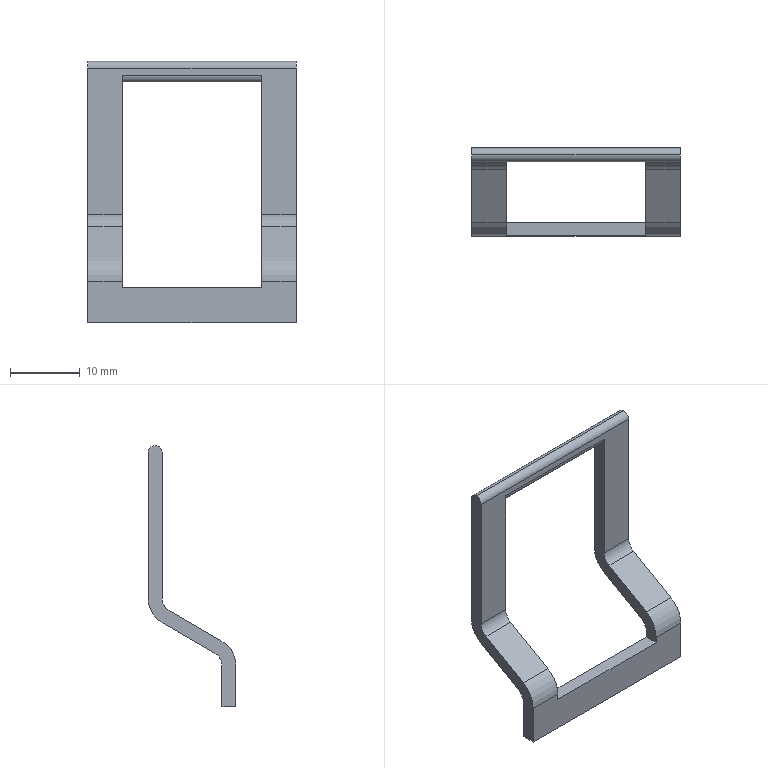Part | SolidWorks | features ICE 9, Draft 2, Fillet 2, Extrusion 1 | 1 solid | 25 faces | box 30 x 12.599 x 37.526 mm | volume 1159 mm3 | plane 14 | cylinder 11 | commonest cylinder face diameters 4 x4 8 x4 2 x3
STEP:
#1=CARTESIAN_POINT('',(0.,-2.,-1.));
#2=VERTEX_POINT('',#1);
#3=CARTESIAN_POINT('',(0.,-1.,0.));
#4=VERTEX_POINT('',#3);
#5=CARTESIAN_POINT('',(0.,-1.,-1.));
#6=DIRECTION('',(-1.,0.,0.));
#7=DIRECTION('',(0.,0.,1.));
#8=AXIS2_PLACEMENT_3D('',#5,#6,#7);
#9=CIRCLE('',#8,1.);
#10=EDGE_CURVE('',#2,#4,#9,.T.);
#11=ORIENTED_EDGE('',*,*,#10,.T.);
#12=CARTESIAN_POINT('',(-30.,-1.,0.));
#13=VERTEX_POINT('',#12);
#14=CARTESIAN_POINT('',(0.,-1.,0.));
#15=DIRECTION('',(-1.,0.,0.));
#16=VECTOR('',#15,1000.);
#17=LINE('',#14,#16);
#18=EDGE_CURVE('',#4,#13,#17,.T.);
#19=ORIENTED_EDGE('',*,*,#18,.T.);
#20=CARTESIAN_POINT('',(-30.,-2.,-1.));
#21=VERTEX_POINT('',#20);
#22=CARTESIAN_POINT('',(-30.,-1.,-1.));
#23=DIRECTION('',(-1.,0.,0.));
#24=DIRECTION('',(0.,0.,1.));
#25=AXIS2_PLACEMENT_3D('',#22,#23,#24);
#26=CIRCLE('',#25,1.);
#27=EDGE_CURVE('',#21,#13,#26,.T.);
#28=ORIENTED_EDGE('',*,*,#27,.F.);
#29=CARTESIAN_POINT('',(0.,-2.,-1.));
#30=DIRECTION('',(-1.,0.,0.));
#31=VECTOR('',#30,1000.);
#32=LINE('',#29,#31);
#33=EDGE_CURVE('',#2,#21,#32,.T.);
#34=ORIENTED_EDGE('',*,*,#33,.F.);
#35=EDGE_LOOP('',(#11,#19,#28,#34));
#36=FACE_OUTER_BOUND('',#35,.T.);
#37=CARTESIAN_POINT('',(0.,-1.,-1.));
#38=DIRECTION('',(-1.,0.,0.));
#39=DIRECTION('',(0.,0.,1.));
#40=AXIS2_PLACEMENT_3D('',#37,#38,#39);
#41=CYLINDRICAL_SURFACE('',#40,1.);
#42=ADVANCED_FACE('',(#36),#41,.T.);
#43=CARTESIAN_POINT('',(-5.,-2.,-2.));
#44=VERTEX_POINT('',#43);
#45=CARTESIAN_POINT('',(-25.,-2.,-2.));
#46=VERTEX_POINT('',#45);
#47=CARTESIAN_POINT('',(0.,-2.,-2.));
#48=DIRECTION('',(-1.,0.,0.));
#49=VECTOR('',#48,1000.);
#50=LINE('',#47,#49);
#51=EDGE_CURVE('',#44,#46,#50,.T.);
#52=ORIENTED_EDGE('',*,*,#51,.T.);
#53=CARTESIAN_POINT('',(-25.,0.,-2.));
#54=VERTEX_POINT('',#53);
#55=CARTESIAN_POINT('',(-25.,-1.,-2.));
#56=DIRECTION('',(-1.,0.,0.));
#57=DIRECTION('',(0.,0.,1.));
#58=AXIS2_PLACEMENT_3D('',#55,#56,#57);
#59=CIRCLE('',#58,1.);
#60=EDGE_CURVE('',#54,#46,#59,.T.);
#61=ORIENTED_EDGE('',*,*,#60,.F.);
#62=CARTESIAN_POINT('',(-5.,0.,-2.));
#63=VERTEX_POINT('',#62);
#64=CARTESIAN_POINT('',(0.,0.,-2.));
#65=DIRECTION('',(-1.,0.,0.));
#66=VECTOR('',#65,1000.);
#67=LINE('',#64,#66);
#68=EDGE_CURVE('',#63,#54,#67,.T.);
#69=ORIENTED_EDGE('',*,*,#68,.F.);
#70=CARTESIAN_POINT('',(-5.,-1.,-2.));
#71=DIRECTION('',(1.,0.,0.));
#72=DIRECTION('',(0.,0.,-1.));
#73=AXIS2_PLACEMENT_3D('',#70,#71,#72);
#74=CIRCLE('',#73,1.);
#75=EDGE_CURVE('',#44,#63,#74,.T.);
#76=ORIENTED_EDGE('',*,*,#75,.F.);
#77=EDGE_LOOP('',(#52,#61,#69,#76));
#78=FACE_OUTER_BOUND('',#77,.T.);
#79=CARTESIAN_POINT('',(0.,-1.,-2.));
#80=DIRECTION('',(-1.,0.,0.));
#81=DIRECTION('',(0.,0.,1.));
#82=AXIS2_PLACEMENT_3D('',#79,#80,#81);
#83=CYLINDRICAL_SURFACE('',#82,1.);
#84=ADVANCED_FACE('',(#78),#83,.T.);
#85=ORIENTED_EDGE('',*,*,#18,.F.);
#86=CARTESIAN_POINT('',(0.,0.,-1.));
#87=VERTEX_POINT('',#86);
#88=CARTESIAN_POINT('',(0.,-1.,-1.));
#89=DIRECTION('',(-1.,0.,0.));
#90=DIRECTION('',(0.,0.,1.));
#91=AXIS2_PLACEMENT_3D('',#88,#89,#90);
#92=CIRCLE('',#91,1.);
#93=EDGE_CURVE('',#4,#87,#92,.T.);
#94=ORIENTED_EDGE('',*,*,#93,.T.);
#95=CARTESIAN_POINT('',(-30.,0.,-1.));
#96=VERTEX_POINT('',#95);
#97=CARTESIAN_POINT('',(0.,0.,-1.));
#98=DIRECTION('',(-1.,0.,0.));
#99=VECTOR('',#98,1000.);
#100=LINE('',#97,#99);
#101=EDGE_CURVE('',#87,#96,#100,.T.);
#102=ORIENTED_EDGE('',*,*,#101,.T.);
#103=CARTESIAN_POINT('',(-30.,-1.,-1.));
#104=DIRECTION('',(-1.,0.,0.));
#105=DIRECTION('',(0.,0.,1.));
#106=AXIS2_PLACEMENT_3D('',#103,#104,#105);
#107=CIRCLE('',#106,1.);
#108=EDGE_CURVE('',#13,#96,#107,.T.);
#109=ORIENTED_EDGE('',*,*,#108,.F.);
#110=EDGE_LOOP('',(#85,#94,#102,#109));
#111=FACE_OUTER_BOUND('',#110,.T.);
#112=CARTESIAN_POINT('',(0.,-1.,-1.));
#113=DIRECTION('',(-1.,0.,0.));
#114=DIRECTION('',(0.,0.,1.));
#115=AXIS2_PLACEMENT_3D('',#112,#113,#114);
#116=CYLINDRICAL_SURFACE('',#115,1.);
#117=ADVANCED_FACE('',(#111),#116,.T.);
#118=CARTESIAN_POINT('',(-30.,-2.,-22.009));
#119=VERTEX_POINT('',#118);
#120=CARTESIAN_POINT('',(-30.,-2.,-2.));
#121=DIRECTION('',(0.,0.,1.));
#122=VECTOR('',#121,1000.);
#123=LINE('',#120,#122);
#124=EDGE_CURVE('',#119,#21,#123,.T.);
#125=ORIENTED_EDGE('',*,*,#124,.F.);
#126=CARTESIAN_POINT('',(-25.,-2.,-22.009));
#127=VERTEX_POINT('',#126);
#128=CARTESIAN_POINT('',(-25.,-2.,-22.009));
#129=DIRECTION('',(1.,0.,0.));
#130=VECTOR('',#129,1000.);
#131=LINE('',#128,#130);
#132=EDGE_CURVE('',#119,#127,#131,.T.);
#133=ORIENTED_EDGE('',*,*,#132,.T.);
#134=CARTESIAN_POINT('',(-25.,-2.,-3.));
#135=DIRECTION('',(0.,0.,1.));
#136=VECTOR('',#135,1000.);
#137=LINE('',#134,#136);
#138=EDGE_CURVE('',#127,#46,#137,.T.);
#139=ORIENTED_EDGE('',*,*,#138,.T.);
#140=ORIENTED_EDGE('',*,*,#51,.F.);
#141=CARTESIAN_POINT('',(-5.,-2.,-22.009));
#142=VERTEX_POINT('',#141);
#143=CARTESIAN_POINT('',(-5.,-2.,-3.));
#144=DIRECTION('',(0.,0.,1.));
#145=VECTOR('',#144,1000.);
#146=LINE('',#143,#145);
#147=EDGE_CURVE('',#142,#44,#146,.T.);
#148=ORIENTED_EDGE('',*,*,#147,.F.);
#149=CARTESIAN_POINT('',(0.,-2.,-22.009));
#150=VERTEX_POINT('',#149);
#151=CARTESIAN_POINT('',(0.,-2.,-22.009));
#152=DIRECTION('',(1.,0.,0.));
#153=VECTOR('',#152,1000.);
#154=LINE('',#151,#153);
#155=EDGE_CURVE('',#142,#150,#154,.T.);
#156=ORIENTED_EDGE('',*,*,#155,.T.);
#157=CARTESIAN_POINT('',(0.,-2.,-2.));
#158=DIRECTION('',(0.,0.,1.));
#159=VECTOR('',#158,1000.);
#160=LINE('',#157,#159);
#161=EDGE_CURVE('',#150,#2,#160,.T.);
#162=ORIENTED_EDGE('',*,*,#161,.T.);
#163=ORIENTED_EDGE('',*,*,#33,.T.);
#164=EDGE_LOOP('',(#125,#133,#139,#140,#148,#156,#162,#163));
#165=FACE_OUTER_BOUND('',#164,.T.);
#166=CARTESIAN_POINT('',(0.,-2.,-2.));
#167=DIRECTION('',(0.,-1.,0.));
#168=DIRECTION('',(0.,0.,-1.));
#169=AXIS2_PLACEMENT_3D('',#166,#167,#168);
#170=PLANE('',#169);
#171=ADVANCED_FACE('',(#165),#170,.T.);
#172=CARTESIAN_POINT('',(-25.,0.,-22.009));
#173=VERTEX_POINT('',#172);
#174=CARTESIAN_POINT('',(-25.,0.,-3.));
#175=DIRECTION('',(0.,0.,1.));
#176=VECTOR('',#175,1000.);
#177=LINE('',#174,#176);
#178=EDGE_CURVE('',#173,#54,#177,.T.);
#179=ORIENTED_EDGE('',*,*,#178,.F.);
#180=CARTESIAN_POINT('',(-30.,0.,-22.009));
#181=VERTEX_POINT('',#180);
#182=CARTESIAN_POINT('',(-30.,0.,-22.009));
#183=DIRECTION('',(-1.,0.,0.));
#184=VECTOR('',#183,1000.);
#185=LINE('',#182,#184);
#186=EDGE_CURVE('',#173,#181,#185,.T.);
#187=ORIENTED_EDGE('',*,*,#186,.T.);
#188=CARTESIAN_POINT('',(-30.,0.,-1.));
#189=DIRECTION('',(0.,0.,-1.));
#190=VECTOR('',#189,1000.);
#191=LINE('',#188,#190);
#192=EDGE_CURVE('',#96,#181,#191,.T.);
#193=ORIENTED_EDGE('',*,*,#192,.F.);
#194=ORIENTED_EDGE('',*,*,#101,.F.);
#195=CARTESIAN_POINT('',(0.,0.,-22.009));
#196=VERTEX_POINT('',#195);
#197=CARTESIAN_POINT('',(0.,0.,-1.));
#198=DIRECTION('',(0.,0.,-1.));
#199=VECTOR('',#198,1000.);
#200=LINE('',#197,#199);
#201=EDGE_CURVE('',#87,#196,#200,.T.);
#202=ORIENTED_EDGE('',*,*,#201,.T.);
#203=CARTESIAN_POINT('',(-5.,0.,-22.009));
#204=VERTEX_POINT('',#203);
#205=CARTESIAN_POINT('',(-5.,0.,-22.009));
#206=DIRECTION('',(-1.,0.,0.));
#207=VECTOR('',#206,1000.);
#208=LINE('',#205,#207);
#209=EDGE_CURVE('',#196,#204,#208,.T.);
#210=ORIENTED_EDGE('',*,*,#209,.T.);
#211=CARTESIAN_POINT('',(-5.,0.,-3.));
#212=DIRECTION('',(0.,0.,1.));
#213=VECTOR('',#212,1000.);
#214=LINE('',#211,#213);
#215=EDGE_CURVE('',#204,#63,#214,.T.);
#216=ORIENTED_EDGE('',*,*,#215,.T.);
#217=ORIENTED_EDGE('',*,*,#68,.T.);
#218=EDGE_LOOP('',(#179,#187,#193,#194,#202,#210,#216,#217));
#219=FACE_OUTER_BOUND('',#218,.T.);
#220=CARTESIAN_POINT('',(0.,0.,-1.));
#221=DIRECTION('',(0.,1.,0.));
#222=DIRECTION('',(0.,0.,1.));
#223=AXIS2_PLACEMENT_3D('',#220,#221,#222);
#224=PLANE('',#223);
#225=ADVANCED_FACE('',(#219),#224,.T.);
#226=CARTESIAN_POINT('',(0.,-2.,-25.473));
#227=VERTEX_POINT('',#226);
#228=CARTESIAN_POINT('',(0.,-9.599,-29.86));
#229=VERTEX_POINT('',#228);
#230=CARTESIAN_POINT('',(0.,0.,-24.318));
#231=DIRECTION('',(0.,-0.866,-0.5));
#232=VECTOR('',#231,1000.);
#233=LINE('',#230,#232);
#234=EDGE_CURVE('',#227,#229,#233,.T.);
#235=ORIENTED_EDGE('',*,*,#234,.F.);
#236=CARTESIAN_POINT('',(0.,-4.,-22.009));
#237=DIRECTION('',(1.,0.,0.));
#238=DIRECTION('',(0.,0.,1.));
#239=AXIS2_PLACEMENT_3D('',#236,#237,#238);
#240=CIRCLE('',#239,4.);
#241=EDGE_CURVE('',#227,#196,#240,.T.);
#242=ORIENTED_EDGE('',*,*,#241,.T.);
#243=ORIENTED_EDGE('',*,*,#201,.F.);
#244=ORIENTED_EDGE('',*,*,#93,.F.);
#245=ORIENTED_EDGE('',*,*,#10,.F.);
#246=ORIENTED_EDGE('',*,*,#161,.F.);
#247=CARTESIAN_POINT('',(0.,-3.,-23.741));
#248=VERTEX_POINT('',#247);
#249=CARTESIAN_POINT('',(0.,-4.,-22.009));
#250=DIRECTION('',(-1.,0.,0.));
#251=DIRECTION('',(0.,0.,1.));
#252=AXIS2_PLACEMENT_3D('',#249,#250,#251);
#253=CIRCLE('',#252,2.);
#254=EDGE_CURVE('',#150,#248,#253,.T.);
#255=ORIENTED_EDGE('',*,*,#254,.T.);
#256=CARTESIAN_POINT('',(0.,-10.599,-28.128));
#257=VERTEX_POINT('',#256);
#258=CARTESIAN_POINT('',(0.,-2.,-23.163));
#259=DIRECTION('',(0.,-0.866,-0.5));
#260=VECTOR('',#259,1000.);
#261=LINE('',#258,#260);
#262=EDGE_CURVE('',#248,#257,#261,.T.);
#263=ORIENTED_EDGE('',*,*,#262,.T.);
#264=CARTESIAN_POINT('',(0.,-12.599,-31.592));
#265=VERTEX_POINT('',#264);
#266=CARTESIAN_POINT('',(0.,-8.599,-31.592));
#267=DIRECTION('',(1.,0.,0.));
#268=DIRECTION('',(0.,0.,1.));
#269=AXIS2_PLACEMENT_3D('',#266,#267,#268);
#270=CIRCLE('',#269,4.);
#271=EDGE_CURVE('',#257,#265,#270,.T.);
#272=ORIENTED_EDGE('',*,*,#271,.T.);
#273=CARTESIAN_POINT('',(0.,-12.599,-37.526));
#274=VERTEX_POINT('',#273);
#275=CARTESIAN_POINT('',(0.,-12.599,-23.163));
#276=DIRECTION('',(0.,0.,1.));
#277=VECTOR('',#276,1000.);
#278=LINE('',#275,#277);
#279=EDGE_CURVE('',#274,#265,#278,.T.);
#280=ORIENTED_EDGE('',*,*,#279,.F.);
#281=CARTESIAN_POINT('',(0.,-10.599,-37.526));
#282=VERTEX_POINT('',#281);
#283=CARTESIAN_POINT('',(0.,-12.599,-37.526));
#284=DIRECTION('',(0.,1.,0.));
#285=VECTOR('',#284,1000.);
#286=LINE('',#283,#285);
#287=EDGE_CURVE('',#274,#282,#286,.T.);
#288=ORIENTED_EDGE('',*,*,#287,.T.);
#289=CARTESIAN_POINT('',(0.,-10.599,-31.592));
#290=VERTEX_POINT('',#289);
#291=CARTESIAN_POINT('',(0.,-10.599,-23.163));
#292=DIRECTION('',(0.,0.,1.));
#293=VECTOR('',#292,1000.);
#294=LINE('',#291,#293);
#295=EDGE_CURVE('',#282,#290,#294,.T.);
#296=ORIENTED_EDGE('',*,*,#295,.T.);
#297=CARTESIAN_POINT('',(0.,-8.599,-31.592));
#298=DIRECTION('',(-1.,0.,0.));
#299=DIRECTION('',(0.,0.,1.));
#300=AXIS2_PLACEMENT_3D('',#297,#298,#299);
#301=CIRCLE('',#300,2.);
#302=EDGE_CURVE('',#290,#229,#301,.T.);
#303=ORIENTED_EDGE('',*,*,#302,.T.);
#304=EDGE_LOOP('',(#235,#242,#243,#244,#245,#246,#255,#263,#272,#280,#288,#296,#303));
#305=FACE_OUTER_BOUND('',#304,.T.);
#306=CARTESIAN_POINT('',(0.,-1.,-1.));
#307=DIRECTION('',(-1.,0.,0.));
#308=DIRECTION('',(0.,0.,1.));
#309=AXIS2_PLACEMENT_3D('',#306,#307,#308);
#310=PLANE('',#309);
#311=ADVANCED_FACE('',(#305),#310,.F.);
#312=ORIENTED_EDGE('',*,*,#192,.T.);
#313=CARTESIAN_POINT('',(-30.,-2.,-25.473));
#314=VERTEX_POINT('',#313);
#315=CARTESIAN_POINT('',(-30.,-4.,-22.009));
#316=DIRECTION('',(-1.,0.,0.));
#317=DIRECTION('',(0.,0.,1.));
#318=AXIS2_PLACEMENT_3D('',#315,#316,#317);
#319=CIRCLE('',#318,4.);
#320=EDGE_CURVE('',#181,#314,#319,.T.);
#321=ORIENTED_EDGE('',*,*,#320,.T.);
#322=CARTESIAN_POINT('',(-30.,-9.599,-29.86));
#323=VERTEX_POINT('',#322);
#324=CARTESIAN_POINT('',(-30.,9.347,-18.922));
#325=DIRECTION('',(0.,0.866,0.5));
#326=VECTOR('',#325,1000.);
#327=LINE('',#324,#326);
#328=EDGE_CURVE('',#323,#314,#327,.T.);
#329=ORIENTED_EDGE('',*,*,#328,.F.);
#330=CARTESIAN_POINT('',(-30.,-10.599,-31.592));
#331=VERTEX_POINT('',#330);
#332=CARTESIAN_POINT('',(-30.,-8.599,-31.592));
#333=DIRECTION('',(1.,0.,0.));
#334=DIRECTION('',(0.,0.,1.));
#335=AXIS2_PLACEMENT_3D('',#332,#333,#334);
#336=CIRCLE('',#335,2.);
#337=EDGE_CURVE('',#323,#331,#336,.T.);
#338=ORIENTED_EDGE('',*,*,#337,.T.);
#339=CARTESIAN_POINT('',(-30.,-10.599,-37.526));
#340=VERTEX_POINT('',#339);
#341=CARTESIAN_POINT('',(-30.,-10.599,-37.526));
#342=DIRECTION('',(0.,0.,-1.));
#343=VECTOR('',#342,1000.);
#344=LINE('',#341,#343);
#345=EDGE_CURVE('',#331,#340,#344,.T.);
#346=ORIENTED_EDGE('',*,*,#345,.T.);
#347=CARTESIAN_POINT('',(-30.,-12.599,-37.526));
#348=VERTEX_POINT('',#347);
#349=CARTESIAN_POINT('',(-30.,-12.599,-37.526));
#350=DIRECTION('',(0.,1.,0.));
#351=VECTOR('',#350,1000.);
#352=LINE('',#349,#351);
#353=EDGE_CURVE('',#348,#340,#352,.T.);
#354=ORIENTED_EDGE('',*,*,#353,.F.);
#355=CARTESIAN_POINT('',(-30.,-12.599,-31.592));
#356=VERTEX_POINT('',#355);
#357=CARTESIAN_POINT('',(-30.,-12.599,-37.526));
#358=DIRECTION('',(0.,0.,-1.));
#359=VECTOR('',#358,1000.);
#360=LINE('',#357,#359);
#361=EDGE_CURVE('',#356,#348,#360,.T.);
#362=ORIENTED_EDGE('',*,*,#361,.F.);
#363=CARTESIAN_POINT('',(-30.,-10.599,-28.128));
#364=VERTEX_POINT('',#363);
#365=CARTESIAN_POINT('',(-30.,-8.599,-31.592));
#366=DIRECTION('',(-1.,0.,0.));
#367=DIRECTION('',(0.,0.,1.));
#368=AXIS2_PLACEMENT_3D('',#365,#366,#367);
#369=CIRCLE('',#368,4.);
#370=EDGE_CURVE('',#356,#364,#369,.T.);
#371=ORIENTED_EDGE('',*,*,#370,.T.);
#372=CARTESIAN_POINT('',(-30.,-3.,-23.741));
#373=VERTEX_POINT('',#372);
#374=CARTESIAN_POINT('',(-30.,8.347,-17.19));
#375=DIRECTION('',(0.,0.866,0.5));
#376=VECTOR('',#375,1000.);
#377=LINE('',#374,#376);
#378=EDGE_CURVE('',#364,#373,#377,.T.);
#379=ORIENTED_EDGE('',*,*,#378,.T.);
#380=CARTESIAN_POINT('',(-30.,-4.,-22.009));
#381=DIRECTION('',(1.,0.,0.));
#382=DIRECTION('',(0.,0.,1.));
#383=AXIS2_PLACEMENT_3D('',#380,#381,#382);
#384=CIRCLE('',#383,2.);
#385=EDGE_CURVE('',#373,#119,#384,.T.);
#386=ORIENTED_EDGE('',*,*,#385,.T.);
#387=ORIENTED_EDGE('',*,*,#124,.T.);
#388=ORIENTED_EDGE('',*,*,#27,.T.);
#389=ORIENTED_EDGE('',*,*,#108,.T.);
#390=EDGE_LOOP('',(#312,#321,#329,#338,#346,#354,#362,#371,#379,#386,#387,#388,#389));
#391=FACE_OUTER_BOUND('',#390,.T.);
#392=CARTESIAN_POINT('',(-30.,-1.,-1.));
#393=DIRECTION('',(-1.,0.,0.));
#394=DIRECTION('',(0.,0.,1.));
#395=AXIS2_PLACEMENT_3D('',#392,#393,#394);
#396=PLANE('',#395);
#397=ADVANCED_FACE('',(#391),#396,.T.);
#398=ORIENTED_EDGE('',*,*,#215,.F.);
#399=CARTESIAN_POINT('',(-5.,-2.,-25.473));
#400=VERTEX_POINT('',#399);
#401=CARTESIAN_POINT('',(-5.,-4.,-22.009));
#402=DIRECTION('',(-1.,0.,0.));
#403=DIRECTION('',(0.,0.,-1.));
#404=AXIS2_PLACEMENT_3D('',#401,#402,#403);
#405=CIRCLE('',#404,4.);
#406=EDGE_CURVE('',#204,#400,#405,.T.);
#407=ORIENTED_EDGE('',*,*,#406,.T.);
#408=CARTESIAN_POINT('',(-5.,-9.599,-29.86));
#409=VERTEX_POINT('',#408);
#410=CARTESIAN_POINT('',(-5.,0.,-24.318));
#411=DIRECTION('',(0.,0.866,0.5));
#412=VECTOR('',#411,1000.);
#413=LINE('',#410,#412);
#414=EDGE_CURVE('',#409,#400,#413,.T.);
#415=ORIENTED_EDGE('',*,*,#414,.F.);
#416=CARTESIAN_POINT('',(-5.,-10.599,-31.592));
#417=VERTEX_POINT('',#416);
#418=CARTESIAN_POINT('',(-5.,-8.599,-31.592));
#419=DIRECTION('',(1.,0.,0.));
#420=DIRECTION('',(0.,0.,-1.));
#421=AXIS2_PLACEMENT_3D('',#418,#419,#420);
#422=CIRCLE('',#421,2.);
#423=EDGE_CURVE('',#409,#417,#422,.T.);
#424=ORIENTED_EDGE('',*,*,#423,.T.);
#425=CARTESIAN_POINT('',(-5.,-10.599,-32.526));
#426=VERTEX_POINT('',#425);
#427=CARTESIAN_POINT('',(-5.,-10.599,-32.526));
#428=DIRECTION('',(0.,0.,-1.));
#429=VECTOR('',#428,1000.);
#430=LINE('',#427,#429);
#431=EDGE_CURVE('',#417,#426,#430,.T.);
#432=ORIENTED_EDGE('',*,*,#431,.T.);
#433=CARTESIAN_POINT('',(-5.,-12.599,-32.526));
#434=VERTEX_POINT('',#433);
#435=CARTESIAN_POINT('',(-5.,-12.599,-32.526));
#436=DIRECTION('',(0.,1.,0.));
#437=VECTOR('',#436,1000.);
#438=LINE('',#435,#437);
#439=EDGE_CURVE('',#434,#426,#438,.T.);
#440=ORIENTED_EDGE('',*,*,#439,.F.);
#441=CARTESIAN_POINT('',(-5.,-12.599,-31.592));
#442=VERTEX_POINT('',#441);
#443=CARTESIAN_POINT('',(-5.,-12.599,-32.526));
#444=DIRECTION('',(0.,0.,-1.));
#445=VECTOR('',#444,1000.);
#446=LINE('',#443,#445);
#447=EDGE_CURVE('',#442,#434,#446,.T.);
#448=ORIENTED_EDGE('',*,*,#447,.F.);
#449=CARTESIAN_POINT('',(-5.,-10.599,-28.128));
#450=VERTEX_POINT('',#449);
#451=CARTESIAN_POINT('',(-5.,-8.599,-31.592));
#452=DIRECTION('',(-1.,0.,0.));
#453=DIRECTION('',(0.,0.,-1.));
#454=AXIS2_PLACEMENT_3D('',#451,#452,#453);
#455=CIRCLE('',#454,4.);
#456=EDGE_CURVE('',#442,#450,#455,.T.);
#457=ORIENTED_EDGE('',*,*,#456,.T.);
#458=CARTESIAN_POINT('',(-5.,-3.,-23.741));
#459=VERTEX_POINT('',#458);
#460=CARTESIAN_POINT('',(-5.,-2.,-23.163));
#461=DIRECTION('',(0.,0.866,0.5));
#462=VECTOR('',#461,1000.);
#463=LINE('',#460,#462);
#464=EDGE_CURVE('',#450,#459,#463,.T.);
#465=ORIENTED_EDGE('',*,*,#464,.T.);
#466=CARTESIAN_POINT('',(-5.,-4.,-22.009));
#467=DIRECTION('',(1.,0.,0.));
#468=DIRECTION('',(0.,0.,-1.));
#469=AXIS2_PLACEMENT_3D('',#466,#467,#468);
#470=CIRCLE('',#469,2.);
#471=EDGE_CURVE('',#459,#142,#470,.T.);
#472=ORIENTED_EDGE('',*,*,#471,.T.);
#473=ORIENTED_EDGE('',*,*,#147,.T.);
#474=ORIENTED_EDGE('',*,*,#75,.T.);
#475=EDGE_LOOP('',(#398,#407,#415,#424,#432,#440,#448,#457,#465,#472,#473,#474));
#476=FACE_OUTER_BOUND('',#475,.T.);
#477=CARTESIAN_POINT('',(-5.,0.,-3.));
#478=DIRECTION('',(1.,0.,0.));
#479=DIRECTION('',(0.,0.,-1.));
#480=AXIS2_PLACEMENT_3D('',#477,#478,#479);
#481=PLANE('',#480);
#482=ADVANCED_FACE('',(#476),#481,.F.);
#483=ORIENTED_EDGE('',*,*,#414,.T.);
#484=CARTESIAN_POINT('',(0.,-2.,-25.473));
#485=DIRECTION('',(1.,0.,0.));
#486=VECTOR('',#485,1000.);
#487=LINE('',#484,#486);
#488=EDGE_CURVE('',#400,#227,#487,.T.);
#489=ORIENTED_EDGE('',*,*,#488,.T.);
#490=ORIENTED_EDGE('',*,*,#234,.T.);
#491=CARTESIAN_POINT('',(0.,-9.599,-29.86));
#492=DIRECTION('',(-1.,0.,0.));
#493=VECTOR('',#492,1000.);
#494=LINE('',#491,#493);
#495=EDGE_CURVE('',#229,#409,#494,.T.);
#496=ORIENTED_EDGE('',*,*,#495,.T.);
#497=EDGE_LOOP('',(#483,#489,#490,#496));
#498=FACE_OUTER_BOUND('',#497,.T.);
#499=CARTESIAN_POINT('',(0.,0.,-24.318));
#500=DIRECTION('',(0.,0.5,-0.866));
#501=DIRECTION('',(0.,0.866,0.5));
#502=AXIS2_PLACEMENT_3D('',#499,#500,#501);
#503=PLANE('',#502);
#504=ADVANCED_FACE('',(#498),#503,.T.);
#505=ORIENTED_EDGE('',*,*,#464,.F.);
#506=CARTESIAN_POINT('',(0.,-10.599,-28.128));
#507=DIRECTION('',(1.,0.,0.));
#508=VECTOR('',#507,1000.);
#509=LINE('',#506,#508);
#510=EDGE_CURVE('',#450,#257,#509,.T.);
#511=ORIENTED_EDGE('',*,*,#510,.T.);
#512=ORIENTED_EDGE('',*,*,#262,.F.);
#513=CARTESIAN_POINT('',(-5.,-3.,-23.741));
#514=DIRECTION('',(-1.,0.,0.));
#515=VECTOR('',#514,1000.);
#516=LINE('',#513,#515);
#517=EDGE_CURVE('',#248,#459,#516,.T.);
#518=ORIENTED_EDGE('',*,*,#517,.T.);
#519=EDGE_LOOP('',(#505,#511,#512,#518));
#520=FACE_OUTER_BOUND('',#519,.T.);
#521=CARTESIAN_POINT('',(-5.,-2.,-23.163));
#522=DIRECTION('',(0.,-0.5,0.866));
#523=DIRECTION('',(0.,-0.866,-0.5));
#524=AXIS2_PLACEMENT_3D('',#521,#522,#523);
#525=PLANE('',#524);
#526=ADVANCED_FACE('',(#520),#525,.T.);
#527=CARTESIAN_POINT('',(-25.,-2.,-25.473));
#528=VERTEX_POINT('',#527);
#529=CARTESIAN_POINT('',(-25.,-9.599,-29.86));
#530=VERTEX_POINT('',#529);
#531=CARTESIAN_POINT('',(-25.,0.,-24.318));
#532=DIRECTION('',(0.,-0.866,-0.5));
#533=VECTOR('',#532,1000.);
#534=LINE('',#531,#533);
#535=EDGE_CURVE('',#528,#530,#534,.T.);
#536=ORIENTED_EDGE('',*,*,#535,.F.);
#537=CARTESIAN_POINT('',(-25.,-4.,-22.009));
#538=DIRECTION('',(1.,0.,0.));
#539=DIRECTION('',(0.,0.,1.));
#540=AXIS2_PLACEMENT_3D('',#537,#538,#539);
#541=CIRCLE('',#540,4.);
#542=EDGE_CURVE('',#528,#173,#541,.T.);
#543=ORIENTED_EDGE('',*,*,#542,.T.);
#544=ORIENTED_EDGE('',*,*,#178,.T.);
#545=ORIENTED_EDGE('',*,*,#60,.T.);
#546=ORIENTED_EDGE('',*,*,#138,.F.);
#547=CARTESIAN_POINT('',(-25.,-3.,-23.741));
#548=VERTEX_POINT('',#547);
#549=CARTESIAN_POINT('',(-25.,-4.,-22.009));
#550=DIRECTION('',(-1.,0.,0.));
#551=DIRECTION('',(0.,0.,1.));
#552=AXIS2_PLACEMENT_3D('',#549,#550,#551);
#553=CIRCLE('',#552,2.);
#554=EDGE_CURVE('',#127,#548,#553,.T.);
#555=ORIENTED_EDGE('',*,*,#554,.T.);
#556=CARTESIAN_POINT('',(-25.,-10.599,-28.128));
#557=VERTEX_POINT('',#556);
#558=CARTESIAN_POINT('',(-25.,-2.,-23.163));
#559=DIRECTION('',(0.,-0.866,-0.5));
#560=VECTOR('',#559,1000.);
#561=LINE('',#558,#560);
#562=EDGE_CURVE('',#548,#557,#561,.T.);
#563=ORIENTED_EDGE('',*,*,#562,.T.);
#564=CARTESIAN_POINT('',(-25.,-12.599,-31.592));
#565=VERTEX_POINT('',#564);
#566=CARTESIAN_POINT('',(-25.,-8.599,-31.592));
#567=DIRECTION('',(1.,0.,0.));
#568=DIRECTION('',(0.,0.,1.));
#569=AXIS2_PLACEMENT_3D('',#566,#567,#568);
#570=CIRCLE('',#569,4.);
#571=EDGE_CURVE('',#557,#565,#570,.T.);
#572=ORIENTED_EDGE('',*,*,#571,.T.);
#573=CARTESIAN_POINT('',(-25.,-12.599,-32.526));
#574=VERTEX_POINT('',#573);
#575=CARTESIAN_POINT('',(-25.,-12.599,-23.163));
#576=DIRECTION('',(0.,0.,1.));
#577=VECTOR('',#576,1000.);
#578=LINE('',#575,#577);
#579=EDGE_CURVE('',#574,#565,#578,.T.);
#580=ORIENTED_EDGE('',*,*,#579,.F.);
#581=CARTESIAN_POINT('',(-25.,-10.599,-32.526));
#582=VERTEX_POINT('',#581);
#583=CARTESIAN_POINT('',(-25.,-12.599,-32.526));
#584=DIRECTION('',(0.,1.,0.));
#585=VECTOR('',#584,1000.);
#586=LINE('',#583,#585);
#587=EDGE_CURVE('',#574,#582,#586,.T.);
#588=ORIENTED_EDGE('',*,*,#587,.T.);
#589=CARTESIAN_POINT('',(-25.,-10.599,-31.592));
#590=VERTEX_POINT('',#589);
#591=CARTESIAN_POINT('',(-25.,-10.599,-23.163));
#592=DIRECTION('',(0.,0.,1.));
#593=VECTOR('',#592,1000.);
#594=LINE('',#591,#593);
#595=EDGE_CURVE('',#582,#590,#594,.T.);
#596=ORIENTED_EDGE('',*,*,#595,.T.);
#597=CARTESIAN_POINT('',(-25.,-8.599,-31.592));
#598=DIRECTION('',(-1.,0.,0.));
#599=DIRECTION('',(0.,0.,1.));
#600=AXIS2_PLACEMENT_3D('',#597,#598,#599);
#601=CIRCLE('',#600,2.);
#602=EDGE_CURVE('',#590,#530,#601,.T.);
#603=ORIENTED_EDGE('',*,*,#602,.T.);
#604=EDGE_LOOP('',(#536,#543,#544,#545,#546,#555,#563,#572,#580,#588,#596,#603));
#605=FACE_OUTER_BOUND('',#604,.T.);
#606=CARTESIAN_POINT('',(-25.,-2.,-3.));
#607=DIRECTION('',(-1.,0.,0.));
#608=DIRECTION('',(0.,0.,1.));
#609=AXIS2_PLACEMENT_3D('',#606,#607,#608);
#610=PLANE('',#609);
#611=ADVANCED_FACE('',(#605),#610,.F.);
#612=ORIENTED_EDGE('',*,*,#328,.T.);
#613=CARTESIAN_POINT('',(-25.,-2.,-25.473));
#614=DIRECTION('',(1.,0.,0.));
#615=VECTOR('',#614,1000.);
#616=LINE('',#613,#615);
#617=EDGE_CURVE('',#314,#528,#616,.T.);
#618=ORIENTED_EDGE('',*,*,#617,.T.);
#619=ORIENTED_EDGE('',*,*,#535,.T.);
#620=CARTESIAN_POINT('',(-25.,-9.599,-29.86));
#621=DIRECTION('',(-1.,0.,0.));
#622=VECTOR('',#621,1000.);
#623=LINE('',#620,#622);
#624=EDGE_CURVE('',#530,#323,#623,.T.);
#625=ORIENTED_EDGE('',*,*,#624,.T.);
#626=EDGE_LOOP('',(#612,#618,#619,#625));
#627=FACE_OUTER_BOUND('',#626,.T.);
#628=CARTESIAN_POINT('',(-25.,0.,-24.318));
#629=DIRECTION('',(0.,0.5,-0.866));
#630=DIRECTION('',(0.,0.866,0.5));
#631=AXIS2_PLACEMENT_3D('',#628,#629,#630);
#632=PLANE('',#631);
#633=ADVANCED_FACE('',(#627),#632,.T.);
#634=ORIENTED_EDGE('',*,*,#378,.F.);
#635=CARTESIAN_POINT('',(-25.,-10.599,-28.128));
#636=DIRECTION('',(1.,0.,0.));
#637=VECTOR('',#636,1000.);
#638=LINE('',#635,#637);
#639=EDGE_CURVE('',#364,#557,#638,.T.);
#640=ORIENTED_EDGE('',*,*,#639,.T.);
#641=ORIENTED_EDGE('',*,*,#562,.F.);
#642=CARTESIAN_POINT('',(-30.,-3.,-23.741));
#643=DIRECTION('',(-1.,0.,0.));
#644=VECTOR('',#643,1000.);
#645=LINE('',#642,#644);
#646=EDGE_CURVE('',#548,#373,#645,.T.);
#647=ORIENTED_EDGE('',*,*,#646,.T.);
#648=EDGE_LOOP('',(#634,#640,#641,#647));
#649=FACE_OUTER_BOUND('',#648,.T.);
#650=CARTESIAN_POINT('',(-30.,-2.,-23.163));
#651=DIRECTION('',(0.,-0.5,0.866));
#652=DIRECTION('',(0.,-0.866,-0.5));
#653=AXIS2_PLACEMENT_3D('',#650,#651,#652);
#654=PLANE('',#653);
#655=ADVANCED_FACE('',(#649),#654,.T.);
#656=ORIENTED_EDGE('',*,*,#345,.F.);
#657=CARTESIAN_POINT('',(0.,-10.599,-31.592));
#658=DIRECTION('',(1.,0.,0.));
#659=VECTOR('',#658,1000.);
#660=LINE('',#657,#659);
#661=EDGE_CURVE('',#331,#590,#660,.T.);
#662=ORIENTED_EDGE('',*,*,#661,.T.);
#663=ORIENTED_EDGE('',*,*,#595,.F.);
#664=CARTESIAN_POINT('',(-25.,-10.599,-32.526));
#665=DIRECTION('',(-1.,0.,0.));
#666=VECTOR('',#665,1000.);
#667=LINE('',#664,#666);
#668=EDGE_CURVE('',#426,#582,#667,.T.);
#669=ORIENTED_EDGE('',*,*,#668,.F.);
#670=ORIENTED_EDGE('',*,*,#431,.F.);
#671=CARTESIAN_POINT('',(0.,-10.599,-31.592));
#672=DIRECTION('',(1.,0.,0.));
#673=VECTOR('',#672,1000.);
#674=LINE('',#671,#673);
#675=EDGE_CURVE('',#417,#290,#674,.T.);
#676=ORIENTED_EDGE('',*,*,#675,.T.);
#677=ORIENTED_EDGE('',*,*,#295,.F.);
#678=CARTESIAN_POINT('',(0.,-10.599,-37.526));
#679=DIRECTION('',(1.,0.,0.));
#680=VECTOR('',#679,1000.);
#681=LINE('',#678,#680);
#682=EDGE_CURVE('',#340,#282,#681,.T.);
#683=ORIENTED_EDGE('',*,*,#682,.F.);
#684=EDGE_LOOP('',(#656,#662,#663,#669,#670,#676,#677,#683));
#685=FACE_OUTER_BOUND('',#684,.T.);
#686=CARTESIAN_POINT('',(0.,-10.599,0.));
#687=DIRECTION('',(0.,1.,0.));
#688=DIRECTION('',(0.,0.,1.));
#689=AXIS2_PLACEMENT_3D('',#686,#687,#688);
#690=PLANE('',#689);
#691=ADVANCED_FACE('',(#685),#690,.T.);
#692=ORIENTED_EDGE('',*,*,#668,.T.);
#693=ORIENTED_EDGE('',*,*,#587,.F.);
#694=CARTESIAN_POINT('',(-25.,-12.599,-32.526));
#695=DIRECTION('',(-1.,0.,0.));
#696=VECTOR('',#695,1000.);
#697=LINE('',#694,#696);
#698=EDGE_CURVE('',#434,#574,#697,.T.);
#699=ORIENTED_EDGE('',*,*,#698,.F.);
#700=ORIENTED_EDGE('',*,*,#439,.T.);
#701=EDGE_LOOP('',(#692,#693,#699,#700));
#702=FACE_OUTER_BOUND('',#701,.T.);
#703=CARTESIAN_POINT('',(-25.,-12.599,-32.526));
#704=DIRECTION('',(0.,0.,-1.));
#705=DIRECTION('',(-1.,0.,0.));
#706=AXIS2_PLACEMENT_3D('',#703,#704,#705);
#707=PLANE('',#706);
#708=ADVANCED_FACE('',(#702),#707,.F.);
#709=ORIENTED_EDGE('',*,*,#682,.T.);
#710=ORIENTED_EDGE('',*,*,#287,.F.);
#711=CARTESIAN_POINT('',(0.,-12.599,-37.526));
#712=DIRECTION('',(1.,0.,0.));
#713=VECTOR('',#712,1000.);
#714=LINE('',#711,#713);
#715=EDGE_CURVE('',#348,#274,#714,.T.);
#716=ORIENTED_EDGE('',*,*,#715,.F.);
#717=ORIENTED_EDGE('',*,*,#353,.T.);
#718=EDGE_LOOP('',(#709,#710,#716,#717));
#719=FACE_OUTER_BOUND('',#718,.T.);
#720=CARTESIAN_POINT('',(0.,-12.599,-37.526));
#721=DIRECTION('',(0.,0.,1.));
#722=DIRECTION('',(1.,0.,0.));
#723=AXIS2_PLACEMENT_3D('',#720,#721,#722);
#724=PLANE('',#723);
#725=ADVANCED_FACE('',(#719),#724,.F.);
#726=ORIENTED_EDGE('',*,*,#279,.T.);
#727=CARTESIAN_POINT('',(-5.,-12.599,-31.592));
#728=DIRECTION('',(-1.,0.,0.));
#729=VECTOR('',#728,1000.);
#730=LINE('',#727,#729);
#731=EDGE_CURVE('',#265,#442,#730,.T.);
#732=ORIENTED_EDGE('',*,*,#731,.T.);
#733=ORIENTED_EDGE('',*,*,#447,.T.);
#734=ORIENTED_EDGE('',*,*,#698,.T.);
#735=ORIENTED_EDGE('',*,*,#579,.T.);
#736=CARTESIAN_POINT('',(-30.,-12.599,-31.592));
#737=DIRECTION('',(-1.,0.,0.));
#738=VECTOR('',#737,1000.);
#739=LINE('',#736,#738);
#740=EDGE_CURVE('',#565,#356,#739,.T.);
#741=ORIENTED_EDGE('',*,*,#740,.T.);
#742=ORIENTED_EDGE('',*,*,#361,.T.);
#743=ORIENTED_EDGE('',*,*,#715,.T.);
#744=EDGE_LOOP('',(#726,#732,#733,#734,#735,#741,#742,#743));
#745=FACE_OUTER_BOUND('',#744,.T.);
#746=CARTESIAN_POINT('',(0.,-12.599,0.));
#747=DIRECTION('',(0.,1.,0.));
#748=DIRECTION('',(0.,0.,1.));
#749=AXIS2_PLACEMENT_3D('',#746,#747,#748);
#750=PLANE('',#749);
#751=ADVANCED_FACE('',(#745),#750,.F.);
#752=ORIENTED_EDGE('',*,*,#554,.F.);
#753=ORIENTED_EDGE('',*,*,#132,.F.);
#754=ORIENTED_EDGE('',*,*,#385,.F.);
#755=ORIENTED_EDGE('',*,*,#646,.F.);
#756=EDGE_LOOP('',(#752,#753,#754,#755));
#757=FACE_OUTER_BOUND('',#756,.T.);
#758=CARTESIAN_POINT('',(-30.,-4.,-22.009));
#759=DIRECTION('',(1.,0.,0.));
#760=DIRECTION('',(0.,0.,-1.));
#761=AXIS2_PLACEMENT_3D('',#758,#759,#760);
#762=CYLINDRICAL_SURFACE('',#761,2.);
#763=ADVANCED_FACE('',(#757),#762,.F.);
#764=ORIENTED_EDGE('',*,*,#254,.F.);
#765=ORIENTED_EDGE('',*,*,#155,.F.);
#766=ORIENTED_EDGE('',*,*,#471,.F.);
#767=ORIENTED_EDGE('',*,*,#517,.F.);
#768=EDGE_LOOP('',(#764,#765,#766,#767));
#769=FACE_OUTER_BOUND('',#768,.T.);
#770=CARTESIAN_POINT('',(-5.,-4.,-22.009));
#771=DIRECTION('',(1.,0.,0.));
#772=DIRECTION('',(0.,0.,-1.));
#773=AXIS2_PLACEMENT_3D('',#770,#771,#772);
#774=CYLINDRICAL_SURFACE('',#773,2.);
#775=ADVANCED_FACE('',(#769),#774,.F.);
#776=ORIENTED_EDGE('',*,*,#602,.F.);
#777=ORIENTED_EDGE('',*,*,#661,.F.);
#778=ORIENTED_EDGE('',*,*,#337,.F.);
#779=ORIENTED_EDGE('',*,*,#624,.F.);
#780=EDGE_LOOP('',(#776,#777,#778,#779));
#781=FACE_OUTER_BOUND('',#780,.T.);
#782=CARTESIAN_POINT('',(-25.,-8.599,-31.592));
#783=DIRECTION('',(1.,0.,0.));
#784=DIRECTION('',(0.,0.,-1.));
#785=AXIS2_PLACEMENT_3D('',#782,#783,#784);
#786=CYLINDRICAL_SURFACE('',#785,2.);
#787=ADVANCED_FACE('',(#781),#786,.F.);
#788=ORIENTED_EDGE('',*,*,#302,.F.);
#789=ORIENTED_EDGE('',*,*,#675,.F.);
#790=ORIENTED_EDGE('',*,*,#423,.F.);
#791=ORIENTED_EDGE('',*,*,#495,.F.);
#792=EDGE_LOOP('',(#788,#789,#790,#791));
#793=FACE_OUTER_BOUND('',#792,.T.);
#794=CARTESIAN_POINT('',(0.,-8.599,-31.592));
#795=DIRECTION('',(1.,0.,0.));
#796=DIRECTION('',(0.,0.,-1.));
#797=AXIS2_PLACEMENT_3D('',#794,#795,#796);
#798=CYLINDRICAL_SURFACE('',#797,2.);
#799=ADVANCED_FACE('',(#793),#798,.F.);
#800=ORIENTED_EDGE('',*,*,#320,.F.);
#801=ORIENTED_EDGE('',*,*,#186,.F.);
#802=ORIENTED_EDGE('',*,*,#542,.F.);
#803=ORIENTED_EDGE('',*,*,#617,.F.);
#804=EDGE_LOOP('',(#800,#801,#802,#803));
#805=FACE_OUTER_BOUND('',#804,.T.);
#806=CARTESIAN_POINT('',(-25.,-4.,-22.009));
#807=DIRECTION('',(1.,0.,0.));
#808=DIRECTION('',(0.,0.,-1.));
#809=AXIS2_PLACEMENT_3D('',#806,#807,#808);
#810=CYLINDRICAL_SURFACE('',#809,4.);
#811=ADVANCED_FACE('',(#805),#810,.T.);
#812=ORIENTED_EDGE('',*,*,#406,.F.);
#813=ORIENTED_EDGE('',*,*,#209,.F.);
#814=ORIENTED_EDGE('',*,*,#241,.F.);
#815=ORIENTED_EDGE('',*,*,#488,.F.);
#816=EDGE_LOOP('',(#812,#813,#814,#815));
#817=FACE_OUTER_BOUND('',#816,.T.);
#818=CARTESIAN_POINT('',(0.,-4.,-22.009));
#819=DIRECTION('',(1.,0.,0.));
#820=DIRECTION('',(0.,0.,-1.));
#821=AXIS2_PLACEMENT_3D('',#818,#819,#820);
#822=CYLINDRICAL_SURFACE('',#821,4.);
#823=ADVANCED_FACE('',(#817),#822,.T.);
#824=ORIENTED_EDGE('',*,*,#271,.F.);
#825=ORIENTED_EDGE('',*,*,#510,.F.);
#826=ORIENTED_EDGE('',*,*,#456,.F.);
#827=ORIENTED_EDGE('',*,*,#731,.F.);
#828=EDGE_LOOP('',(#824,#825,#826,#827));
#829=FACE_OUTER_BOUND('',#828,.T.);
#830=CARTESIAN_POINT('',(0.,-8.599,-31.592));
#831=DIRECTION('',(1.,0.,0.));
#832=DIRECTION('',(0.,0.,-1.));
#833=AXIS2_PLACEMENT_3D('',#830,#831,#832);
#834=CYLINDRICAL_SURFACE('',#833,4.);
#835=ADVANCED_FACE('',(#829),#834,.T.);
#836=ORIENTED_EDGE('',*,*,#571,.F.);
#837=ORIENTED_EDGE('',*,*,#639,.F.);
#838=ORIENTED_EDGE('',*,*,#370,.F.);
#839=ORIENTED_EDGE('',*,*,#740,.F.);
#840=EDGE_LOOP('',(#836,#837,#838,#839));
#841=FACE_OUTER_BOUND('',#840,.T.);
#842=CARTESIAN_POINT('',(0.,-8.599,-31.592));
#843=DIRECTION('',(1.,0.,0.));
#844=DIRECTION('',(0.,0.,-1.));
#845=AXIS2_PLACEMENT_3D('',#842,#843,#844);
#846=CYLINDRICAL_SURFACE('',#845,4.);
#847=ADVANCED_FACE('',(#841),#846,.T.);
#848=CLOSED_SHELL('',(#42,#84,#117,#171,#225,#311,#397,#482,#504,#526,#611,#633,#655,#691,#708,#725,#751,#763,#775,#787,#799,#811,#823,#835,#847));
#849=MANIFOLD_SOLID_BREP('',#848);
#850=CARTESIAN_POINT('',(0.,0.,0.));
#851=DIRECTION('',(0.,0.,1.));
#852=DIRECTION('',(1.,0.,0.));
#853=AXIS2_PLACEMENT_3D('',#850,#851,#852);
#854=(LENGTH_UNIT()NAMED_UNIT(*)SI_UNIT(.MILLI.,.METRE.));
#855=UNCERTAINTY_MEASURE_WITH_UNIT(LENGTH_MEASURE(0.00001),#854,'','');
#856=(NAMED_UNIT(*)PLANE_ANGLE_UNIT()SI_UNIT($,.RADIAN.));
#857=(NAMED_UNIT(*)SI_UNIT($,.STERADIAN.)SOLID_ANGLE_UNIT());
#858=(GEOMETRIC_REPRESENTATION_CONTEXT(3)GLOBAL_UNCERTAINTY_ASSIGNED_CONTEXT((#855))GLOBAL_UNIT_ASSIGNED_CONTEXT((#854,#856,#857))REPRESENTATION_CONTEXT('',''));
#859=ADVANCED_BREP_SHAPE_REPRESENTATION('',(#849,#853),#858);